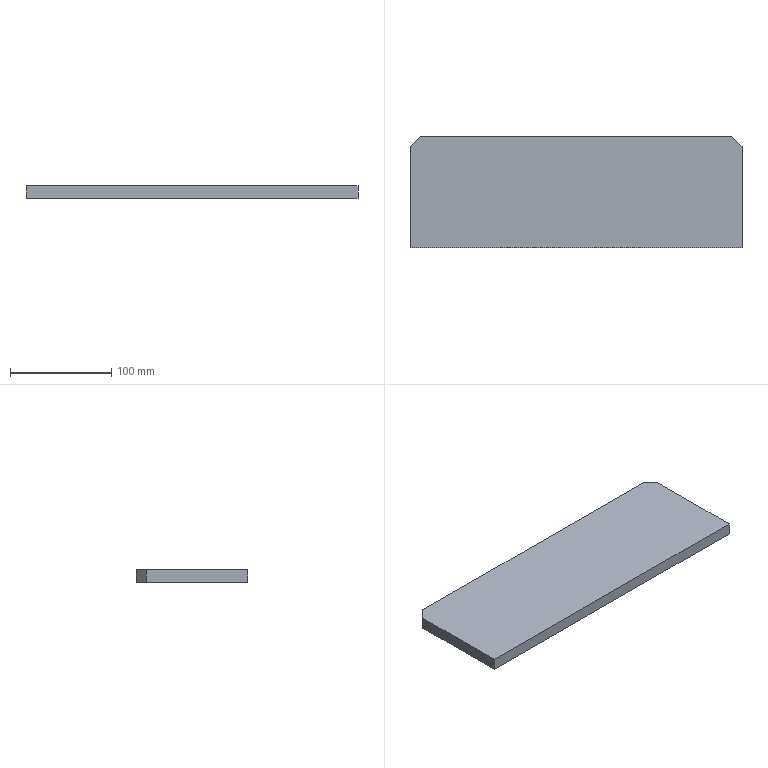Part | SolidWorks | features BaseBody 1 | 1 solid | 8 faces | box 328 x 110 x 12 mm | volume 431760 mm3 | plane 8
STEP:
#1=CARTESIAN_POINT('',(164.,-55.,0.));
#2=VERTEX_POINT('',#1);
#3=CARTESIAN_POINT('',(164.,45.,0.));
#4=VERTEX_POINT('',#3);
#5=CARTESIAN_POINT('',(164.,45.,0.));
#6=DIRECTION('',(0.,1.,0.));
#7=VECTOR('',#6,1000.);
#8=LINE('',#5,#7);
#9=EDGE_CURVE('',#2,#4,#8,.T.);
#10=ORIENTED_EDGE('',*,*,#9,.T.);
#11=CARTESIAN_POINT('',(164.,45.,12.));
#12=VERTEX_POINT('',#11);
#13=CARTESIAN_POINT('',(164.,45.,12.));
#14=DIRECTION('',(0.,0.,-1.));
#15=VECTOR('',#14,1000.);
#16=LINE('',#13,#15);
#17=EDGE_CURVE('',#12,#4,#16,.T.);
#18=ORIENTED_EDGE('',*,*,#17,.F.);
#19=CARTESIAN_POINT('',(164.,-55.,12.));
#20=VERTEX_POINT('',#19);
#21=CARTESIAN_POINT('',(164.,45.,12.));
#22=DIRECTION('',(0.,1.,0.));
#23=VECTOR('',#22,1000.);
#24=LINE('',#21,#23);
#25=EDGE_CURVE('',#20,#12,#24,.T.);
#26=ORIENTED_EDGE('',*,*,#25,.F.);
#27=CARTESIAN_POINT('',(164.,-55.,12.));
#28=DIRECTION('',(0.,0.,-1.));
#29=VECTOR('',#28,1000.);
#30=LINE('',#27,#29);
#31=EDGE_CURVE('',#20,#2,#30,.T.);
#32=ORIENTED_EDGE('',*,*,#31,.T.);
#33=EDGE_LOOP('',(#10,#18,#26,#32));
#34=FACE_OUTER_BOUND('',#33,.T.);
#35=CARTESIAN_POINT('',(164.,45.,12.));
#36=DIRECTION('',(-1.,0.,0.));
#37=DIRECTION('',(0.,0.,1.));
#38=AXIS2_PLACEMENT_3D('',#35,#36,#37);
#39=PLANE('',#38);
#40=ADVANCED_FACE('',(#34),#39,.F.);
#41=CARTESIAN_POINT('',(154.,55.,0.));
#42=VERTEX_POINT('',#41);
#43=CARTESIAN_POINT('',(154.,55.,0.));
#44=DIRECTION('',(-0.7071,0.7071,0.));
#45=VECTOR('',#44,1000.);
#46=LINE('',#43,#45);
#47=EDGE_CURVE('',#4,#42,#46,.T.);
#48=ORIENTED_EDGE('',*,*,#47,.T.);
#49=CARTESIAN_POINT('',(154.,55.,12.));
#50=VERTEX_POINT('',#49);
#51=CARTESIAN_POINT('',(154.,55.,12.));
#52=DIRECTION('',(0.,0.,-1.));
#53=VECTOR('',#52,1000.);
#54=LINE('',#51,#53);
#55=EDGE_CURVE('',#50,#42,#54,.T.);
#56=ORIENTED_EDGE('',*,*,#55,.F.);
#57=CARTESIAN_POINT('',(154.,55.,12.));
#58=DIRECTION('',(-0.7071,0.7071,0.));
#59=VECTOR('',#58,1000.);
#60=LINE('',#57,#59);
#61=EDGE_CURVE('',#12,#50,#60,.T.);
#62=ORIENTED_EDGE('',*,*,#61,.F.);
#63=ORIENTED_EDGE('',*,*,#17,.T.);
#64=EDGE_LOOP('',(#48,#56,#62,#63));
#65=FACE_OUTER_BOUND('',#64,.T.);
#66=CARTESIAN_POINT('',(154.,55.,12.));
#67=DIRECTION('',(-0.7071,-0.7071,0.));
#68=DIRECTION('',(0.7071,-0.7071,0.));
#69=AXIS2_PLACEMENT_3D('',#66,#67,#68);
#70=PLANE('',#69);
#71=ADVANCED_FACE('',(#65),#70,.F.);
#72=CARTESIAN_POINT('',(-154.,55.,0.));
#73=VERTEX_POINT('',#72);
#74=CARTESIAN_POINT('',(-154.,55.,0.));
#75=DIRECTION('',(-1.,0.,0.));
#76=VECTOR('',#75,1000.);
#77=LINE('',#74,#76);
#78=EDGE_CURVE('',#42,#73,#77,.T.);
#79=ORIENTED_EDGE('',*,*,#78,.T.);
#80=CARTESIAN_POINT('',(-154.,55.,12.));
#81=VERTEX_POINT('',#80);
#82=CARTESIAN_POINT('',(-154.,55.,12.));
#83=DIRECTION('',(0.,0.,-1.));
#84=VECTOR('',#83,1000.);
#85=LINE('',#82,#84);
#86=EDGE_CURVE('',#81,#73,#85,.T.);
#87=ORIENTED_EDGE('',*,*,#86,.F.);
#88=CARTESIAN_POINT('',(-154.,55.,12.));
#89=DIRECTION('',(-1.,0.,0.));
#90=VECTOR('',#89,1000.);
#91=LINE('',#88,#90);
#92=EDGE_CURVE('',#50,#81,#91,.T.);
#93=ORIENTED_EDGE('',*,*,#92,.F.);
#94=ORIENTED_EDGE('',*,*,#55,.T.);
#95=EDGE_LOOP('',(#79,#87,#93,#94));
#96=FACE_OUTER_BOUND('',#95,.T.);
#97=CARTESIAN_POINT('',(-154.,55.,12.));
#98=DIRECTION('',(0.,-1.,0.));
#99=DIRECTION('',(0.,0.,-1.));
#100=AXIS2_PLACEMENT_3D('',#97,#98,#99);
#101=PLANE('',#100);
#102=ADVANCED_FACE('',(#96),#101,.F.);
#103=CARTESIAN_POINT('',(-164.,45.,0.));
#104=VERTEX_POINT('',#103);
#105=CARTESIAN_POINT('',(-164.,45.,0.));
#106=DIRECTION('',(-0.7071,-0.7071,0.));
#107=VECTOR('',#106,1000.);
#108=LINE('',#105,#107);
#109=EDGE_CURVE('',#73,#104,#108,.T.);
#110=ORIENTED_EDGE('',*,*,#109,.T.);
#111=CARTESIAN_POINT('',(-164.,45.,12.));
#112=VERTEX_POINT('',#111);
#113=CARTESIAN_POINT('',(-164.,45.,12.));
#114=DIRECTION('',(0.,0.,-1.));
#115=VECTOR('',#114,1000.);
#116=LINE('',#113,#115);
#117=EDGE_CURVE('',#112,#104,#116,.T.);
#118=ORIENTED_EDGE('',*,*,#117,.F.);
#119=CARTESIAN_POINT('',(-164.,45.,12.));
#120=DIRECTION('',(-0.7071,-0.7071,0.));
#121=VECTOR('',#120,1000.);
#122=LINE('',#119,#121);
#123=EDGE_CURVE('',#81,#112,#122,.T.);
#124=ORIENTED_EDGE('',*,*,#123,.F.);
#125=ORIENTED_EDGE('',*,*,#86,.T.);
#126=EDGE_LOOP('',(#110,#118,#124,#125));
#127=FACE_OUTER_BOUND('',#126,.T.);
#128=CARTESIAN_POINT('',(-164.,45.,12.));
#129=DIRECTION('',(0.7071,-0.7071,0.));
#130=DIRECTION('',(0.7071,0.7071,0.));
#131=AXIS2_PLACEMENT_3D('',#128,#129,#130);
#132=PLANE('',#131);
#133=ADVANCED_FACE('',(#127),#132,.F.);
#134=CARTESIAN_POINT('',(-164.,-55.,0.));
#135=VERTEX_POINT('',#134);
#136=CARTESIAN_POINT('',(-164.,45.,0.));
#137=DIRECTION('',(0.,-1.,0.));
#138=VECTOR('',#137,1000.);
#139=LINE('',#136,#138);
#140=EDGE_CURVE('',#104,#135,#139,.T.);
#141=ORIENTED_EDGE('',*,*,#140,.T.);
#142=CARTESIAN_POINT('',(-164.,-55.,12.));
#143=VERTEX_POINT('',#142);
#144=CARTESIAN_POINT('',(-164.,-55.,12.));
#145=DIRECTION('',(0.,0.,-1.));
#146=VECTOR('',#145,1000.);
#147=LINE('',#144,#146);
#148=EDGE_CURVE('',#143,#135,#147,.T.);
#149=ORIENTED_EDGE('',*,*,#148,.F.);
#150=CARTESIAN_POINT('',(-164.,45.,12.));
#151=DIRECTION('',(0.,-1.,0.));
#152=VECTOR('',#151,1000.);
#153=LINE('',#150,#152);
#154=EDGE_CURVE('',#112,#143,#153,.T.);
#155=ORIENTED_EDGE('',*,*,#154,.F.);
#156=ORIENTED_EDGE('',*,*,#117,.T.);
#157=EDGE_LOOP('',(#141,#149,#155,#156));
#158=FACE_OUTER_BOUND('',#157,.T.);
#159=CARTESIAN_POINT('',(-164.,45.,12.));
#160=DIRECTION('',(1.,0.,0.));
#161=DIRECTION('',(0.,1.,0.));
#162=AXIS2_PLACEMENT_3D('',#159,#160,#161);
#163=PLANE('',#162);
#164=ADVANCED_FACE('',(#158),#163,.F.);
#165=CARTESIAN_POINT('',(-164.,-55.,0.));
#166=DIRECTION('',(1.,0.,0.));
#167=VECTOR('',#166,1000.);
#168=LINE('',#165,#167);
#169=EDGE_CURVE('',#135,#2,#168,.T.);
#170=ORIENTED_EDGE('',*,*,#169,.T.);
#171=ORIENTED_EDGE('',*,*,#31,.F.);
#172=CARTESIAN_POINT('',(-164.,-55.,12.));
#173=DIRECTION('',(1.,0.,0.));
#174=VECTOR('',#173,1000.);
#175=LINE('',#172,#174);
#176=EDGE_CURVE('',#143,#20,#175,.T.);
#177=ORIENTED_EDGE('',*,*,#176,.F.);
#178=ORIENTED_EDGE('',*,*,#148,.T.);
#179=EDGE_LOOP('',(#170,#171,#177,#178));
#180=FACE_OUTER_BOUND('',#179,.T.);
#181=CARTESIAN_POINT('',(-164.,-55.,12.));
#182=DIRECTION('',(0.,1.,0.));
#183=DIRECTION('',(0.,0.,1.));
#184=AXIS2_PLACEMENT_3D('',#181,#182,#183);
#185=PLANE('',#184);
#186=ADVANCED_FACE('',(#180),#185,.F.);
#187=ORIENTED_EDGE('',*,*,#25,.T.);
#188=ORIENTED_EDGE('',*,*,#61,.T.);
#189=ORIENTED_EDGE('',*,*,#92,.T.);
#190=ORIENTED_EDGE('',*,*,#123,.T.);
#191=ORIENTED_EDGE('',*,*,#154,.T.);
#192=ORIENTED_EDGE('',*,*,#176,.T.);
#193=EDGE_LOOP('',(#187,#188,#189,#190,#191,#192));
#194=FACE_OUTER_BOUND('',#193,.T.);
#195=CARTESIAN_POINT('',(0.,0.,12.));
#196=DIRECTION('',(0.,0.,1.));
#197=DIRECTION('',(1.,0.,0.));
#198=AXIS2_PLACEMENT_3D('',#195,#196,#197);
#199=PLANE('',#198);
#200=ADVANCED_FACE('',(#194),#199,.T.);
#201=ORIENTED_EDGE('',*,*,#9,.F.);
#202=ORIENTED_EDGE('',*,*,#169,.F.);
#203=ORIENTED_EDGE('',*,*,#140,.F.);
#204=ORIENTED_EDGE('',*,*,#109,.F.);
#205=ORIENTED_EDGE('',*,*,#78,.F.);
#206=ORIENTED_EDGE('',*,*,#47,.F.);
#207=EDGE_LOOP('',(#201,#202,#203,#204,#205,#206));
#208=FACE_OUTER_BOUND('',#207,.T.);
#209=CARTESIAN_POINT('',(0.,0.,0.));
#210=DIRECTION('',(0.,0.,1.));
#211=DIRECTION('',(1.,0.,0.));
#212=AXIS2_PLACEMENT_3D('',#209,#210,#211);
#213=PLANE('',#212);
#214=ADVANCED_FACE('',(#208),#213,.F.);
#215=CLOSED_SHELL('',(#40,#71,#102,#133,#164,#186,#200,#214));
#216=MANIFOLD_SOLID_BREP('',#215);
#217=CARTESIAN_POINT('',(0.,0.,0.));
#218=DIRECTION('',(0.,0.,1.));
#219=DIRECTION('',(1.,0.,0.));
#220=AXIS2_PLACEMENT_3D('',#217,#218,#219);
#221=(LENGTH_UNIT()NAMED_UNIT(*)SI_UNIT(.MILLI.,.METRE.));
#222=UNCERTAINTY_MEASURE_WITH_UNIT(LENGTH_MEASURE(0.00001),#221,'','');
#223=(NAMED_UNIT(*)PLANE_ANGLE_UNIT()SI_UNIT($,.RADIAN.));
#224=(NAMED_UNIT(*)SI_UNIT($,.STERADIAN.)SOLID_ANGLE_UNIT());
#225=(GEOMETRIC_REPRESENTATION_CONTEXT(3)GLOBAL_UNCERTAINTY_ASSIGNED_CONTEXT((#222))GLOBAL_UNIT_ASSIGNED_CONTEXT((#221,#223,#224))REPRESENTATION_CONTEXT('',''));
#226=ADVANCED_BREP_SHAPE_REPRESENTATION('',(#216,#220),#225);